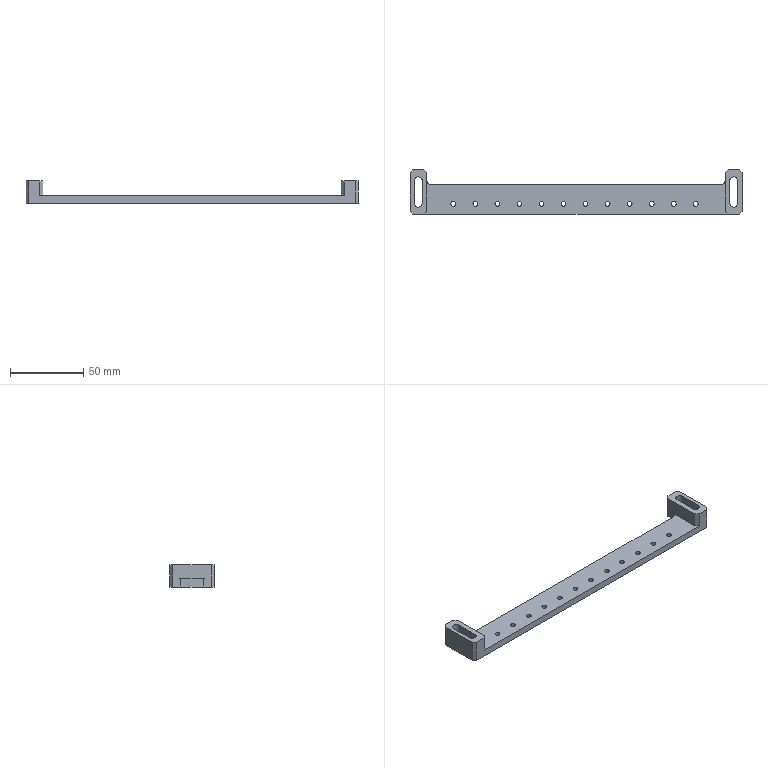Part | SolidWorks | features ICE 4, Chamfer 1, Extrusion 1, Fillet 1, HoleWzd 1, LPattern 1 | 1 solid | 64 faces | box 226 x 30 x 15 mm | volume 25281 mm3 | cylinder 34 | plane 30 | commonest cylinder face diameters 3.3 x24 5.5 x4 10 x4 6 x2